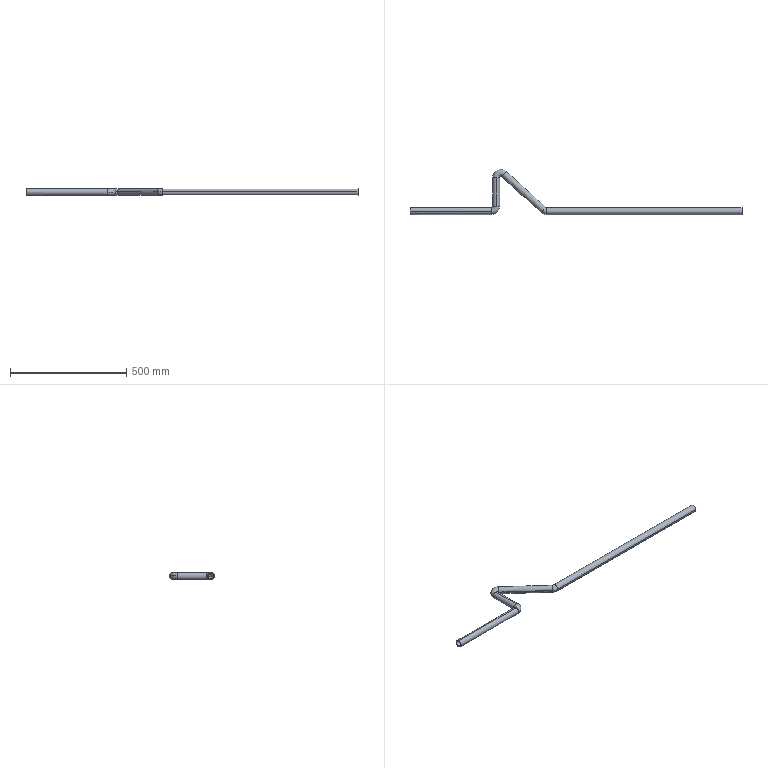Part | SolidWorks | features 3DProfileFeature 2, Sweep 1 | 1 solid | 30 faces | box 1430 x 195.048 x 30 mm | volume 288468 mm3 | cylinder 16 | torus 12 | plane 2 | commonest cylinder face diameters 26 x8 30 x8
STEP:
#1=CARTESIAN_POINT('',(-1540.71,3149.368,100.));
#2=VERTEX_POINT('',#1);
#3=CARTESIAN_POINT('',(-1558.147,3130.082,100.));
#4=VERTEX_POINT('',#3);
#5=CARTESIAN_POINT('',(-1549.428,3139.725,100.));
#6=DIRECTION('',(-0.7418,0.6707,0.));
#7=DIRECTION('',(0.6707,0.7418,0.));
#8=AXIS2_PLACEMENT_3D('',#5,#6,#7);
#9=CIRCLE('',#8,13.);
#10=EDGE_CURVE('',#2,#4,#9,.T.);
#11=ORIENTED_EDGE('',*,*,#10,.T.);
#12=CARTESIAN_POINT('',(-1536.015,3121.56,100.));
#13=VERTEX_POINT('',#12);
#14=CARTESIAN_POINT('',(-1536.015,3154.56,100.));
#15=DIRECTION('',(0.,0.,1.));
#16=DIRECTION('',(0.,-1.,0.));
#17=AXIS2_PLACEMENT_3D('',#14,#15,#16);
#18=CIRCLE('',#17,33.);
#19=EDGE_CURVE('',#4,#13,#18,.T.);
#20=ORIENTED_EDGE('',*,*,#19,.T.);
#21=CARTESIAN_POINT('',(-1536.015,3147.56,100.));
#22=VERTEX_POINT('',#21);
#23=CARTESIAN_POINT('',(-1536.015,3134.56,100.));
#24=DIRECTION('',(-1.,0.,0.));
#25=DIRECTION('',(0.,-1.,0.));
#26=AXIS2_PLACEMENT_3D('',#23,#24,#25);
#27=CIRCLE('',#26,13.);
#28=EDGE_CURVE('',#22,#13,#27,.T.);
#29=ORIENTED_EDGE('',*,*,#28,.F.);
#30=CARTESIAN_POINT('',(-1536.015,3154.56,100.));
#31=DIRECTION('',(0.,0.,1.));
#32=DIRECTION('',(0.,-1.,0.));
#33=AXIS2_PLACEMENT_3D('',#30,#31,#32);
#34=CIRCLE('',#33,7.);
#35=EDGE_CURVE('',#2,#22,#34,.T.);
#36=ORIENTED_EDGE('',*,*,#35,.F.);
#37=EDGE_LOOP('',(#11,#20,#29,#36));
#38=FACE_OUTER_BOUND('',#37,.T.);
#39=CARTESIAN_POINT('',(-1536.015,3154.56,100.));
#40=DIRECTION('',(0.,0.,1.));
#41=DIRECTION('',(0.,-1.,0.));
#42=AXIS2_PLACEMENT_3D('',#39,#40,#41);
#43=TOROIDAL_SURFACE('',#42,20.,13.);
#44=ADVANCED_FACE('',(#38),#43,.F.);
#45=CARTESIAN_POINT('',(-1753.961,3279.608,113.));
#46=VERTEX_POINT('',#45);
#47=CARTESIAN_POINT('',(-1766.961,3279.608,100.));
#48=VERTEX_POINT('',#47);
#49=CARTESIAN_POINT('',(-1753.961,3279.608,100.));
#50=DIRECTION('',(0.,-1.,0.));
#51=DIRECTION('',(0.,0.,1.));
#52=AXIS2_PLACEMENT_3D('',#49,#50,#51);
#53=CIRCLE('',#52,13.);
#54=EDGE_CURVE('',#46,#48,#53,.T.);
#55=ORIENTED_EDGE('',*,*,#54,.T.);
#56=CARTESIAN_POINT('',(-1711.829,3304.086,100.));
#57=VERTEX_POINT('',#56);
#58=CARTESIAN_POINT('',(-1733.961,3279.608,100.));
#59=DIRECTION('',(0.,0.,-1.));
#60=DIRECTION('',(-1.,0.,0.));
#61=AXIS2_PLACEMENT_3D('',#58,#59,#60);
#62=CIRCLE('',#61,33.);
#63=EDGE_CURVE('',#48,#57,#62,.T.);
#64=ORIENTED_EDGE('',*,*,#63,.T.);
#65=CARTESIAN_POINT('',(-1729.266,3284.801,100.));
#66=VERTEX_POINT('',#65);
#67=CARTESIAN_POINT('',(-1720.547,3294.443,100.));
#68=DIRECTION('',(-0.7418,0.6707,0.));
#69=DIRECTION('',(-0.6707,-0.7418,0.));
#70=AXIS2_PLACEMENT_3D('',#67,#68,#69);
#71=CIRCLE('',#70,13.);
#72=EDGE_CURVE('',#66,#57,#71,.T.);
#73=ORIENTED_EDGE('',*,*,#72,.F.);
#74=CARTESIAN_POINT('',(-1740.961,3279.608,100.));
#75=VERTEX_POINT('',#74);
#76=CARTESIAN_POINT('',(-1733.961,3279.608,100.));
#77=DIRECTION('',(0.,0.,-1.));
#78=DIRECTION('',(-1.,0.,0.));
#79=AXIS2_PLACEMENT_3D('',#76,#77,#78);
#80=CIRCLE('',#79,7.);
#81=EDGE_CURVE('',#75,#66,#80,.T.);
#82=ORIENTED_EDGE('',*,*,#81,.F.);
#83=CARTESIAN_POINT('',(-1753.961,3279.608,100.));
#84=DIRECTION('',(0.,-1.,0.));
#85=DIRECTION('',(0.,0.,1.));
#86=AXIS2_PLACEMENT_3D('',#83,#84,#85);
#87=CIRCLE('',#86,13.);
#88=EDGE_CURVE('',#75,#46,#87,.T.);
#89=ORIENTED_EDGE('',*,*,#88,.T.);
#90=EDGE_LOOP('',(#55,#64,#73,#82,#89));
#91=FACE_OUTER_BOUND('',#90,.T.);
#92=CARTESIAN_POINT('',(-1733.961,3279.608,100.));
#93=DIRECTION('',(0.,0.,-1.));
#94=DIRECTION('',(-1.,0.,0.));
#95=AXIS2_PLACEMENT_3D('',#92,#93,#94);
#96=TOROIDAL_SURFACE('',#95,20.,13.);
#97=ADVANCED_FACE('',(#91),#96,.F.);
#98=CARTESIAN_POINT('',(-1773.961,3135.003,87.));
#99=VERTEX_POINT('',#98);
#100=CARTESIAN_POINT('',(-1773.961,3122.003,100.));
#101=VERTEX_POINT('',#100);
#102=CARTESIAN_POINT('',(-1773.961,3135.003,100.));
#103=DIRECTION('',(-1.,0.,0.));
#104=DIRECTION('',(0.,0.,-1.));
#105=AXIS2_PLACEMENT_3D('',#102,#103,#104);
#106=CIRCLE('',#105,13.);
#107=EDGE_CURVE('',#99,#101,#106,.T.);
#108=ORIENTED_EDGE('',*,*,#107,.T.);
#109=CARTESIAN_POINT('',(-1740.961,3155.003,100.));
#110=VERTEX_POINT('',#109);
#111=CARTESIAN_POINT('',(-1773.961,3155.003,100.));
#112=DIRECTION('',(0.,0.,1.));
#113=DIRECTION('',(1.,0.,0.));
#114=AXIS2_PLACEMENT_3D('',#111,#112,#113);
#115=CIRCLE('',#114,33.);
#116=EDGE_CURVE('',#101,#110,#115,.T.);
#117=ORIENTED_EDGE('',*,*,#116,.T.);
#118=CARTESIAN_POINT('',(-1753.961,3155.003,87.));
#119=VERTEX_POINT('',#118);
#120=CARTESIAN_POINT('',(-1753.961,3155.003,100.));
#121=DIRECTION('',(0.,-1.,0.));
#122=DIRECTION('',(0.,0.,-1.));
#123=AXIS2_PLACEMENT_3D('',#120,#121,#122);
#124=CIRCLE('',#123,13.);
#125=EDGE_CURVE('',#119,#110,#124,.T.);
#126=ORIENTED_EDGE('',*,*,#125,.F.);
#127=CARTESIAN_POINT('',(-1766.961,3155.003,100.));
#128=VERTEX_POINT('',#127);
#129=CARTESIAN_POINT('',(-1753.961,3155.003,100.));
#130=DIRECTION('',(0.,-1.,0.));
#131=DIRECTION('',(0.,0.,-1.));
#132=AXIS2_PLACEMENT_3D('',#129,#130,#131);
#133=CIRCLE('',#132,13.);
#134=EDGE_CURVE('',#128,#119,#133,.T.);
#135=ORIENTED_EDGE('',*,*,#134,.F.);
#136=CARTESIAN_POINT('',(-1773.961,3148.003,100.));
#137=VERTEX_POINT('',#136);
#138=CARTESIAN_POINT('',(-1773.961,3155.003,100.));
#139=DIRECTION('',(0.,0.,1.));
#140=DIRECTION('',(1.,0.,0.));
#141=AXIS2_PLACEMENT_3D('',#138,#139,#140);
#142=CIRCLE('',#141,7.);
#143=EDGE_CURVE('',#137,#128,#142,.T.);
#144=ORIENTED_EDGE('',*,*,#143,.F.);
#145=CARTESIAN_POINT('',(-1773.961,3135.003,100.));
#146=DIRECTION('',(-1.,0.,0.));
#147=DIRECTION('',(0.,0.,-1.));
#148=AXIS2_PLACEMENT_3D('',#145,#146,#147);
#149=CIRCLE('',#148,13.);
#150=EDGE_CURVE('',#137,#99,#149,.T.);
#151=ORIENTED_EDGE('',*,*,#150,.T.);
#152=EDGE_LOOP('',(#108,#117,#126,#135,#144,#151));
#153=FACE_OUTER_BOUND('',#152,.T.);
#154=CARTESIAN_POINT('',(-1773.961,3155.003,100.));
#155=DIRECTION('',(0.,0.,1.));
#156=DIRECTION('',(1.,0.,0.));
#157=AXIS2_PLACEMENT_3D('',#154,#155,#156);
#158=TOROIDAL_SURFACE('',#157,20.,13.);
#159=ADVANCED_FACE('',(#153),#158,.F.);
#160=CARTESIAN_POINT('',(-1559.488,3128.598,100.));
#161=VERTEX_POINT('',#160);
#162=CARTESIAN_POINT('',(-1539.368,3150.851,100.));
#163=VERTEX_POINT('',#162);
#164=CARTESIAN_POINT('',(-1549.428,3139.725,100.));
#165=DIRECTION('',(-0.7418,0.6707,0.));
#166=DIRECTION('',(0.,0.,1.));
#167=AXIS2_PLACEMENT_3D('',#164,#165,#166);
#168=CIRCLE('',#167,15.);
#169=EDGE_CURVE('',#161,#163,#168,.T.);
#170=ORIENTED_EDGE('',*,*,#169,.F.);
#171=CARTESIAN_POINT('',(-1536.015,3119.56,100.));
#172=VERTEX_POINT('',#171);
#173=CARTESIAN_POINT('',(-1536.015,3154.56,100.));
#174=DIRECTION('',(0.,0.,1.));
#175=DIRECTION('',(0.,-1.,0.));
#176=AXIS2_PLACEMENT_3D('',#173,#174,#175);
#177=CIRCLE('',#176,35.);
#178=EDGE_CURVE('',#161,#172,#177,.T.);
#179=ORIENTED_EDGE('',*,*,#178,.T.);
#180=CARTESIAN_POINT('',(-1536.015,3149.56,100.));
#181=VERTEX_POINT('',#180);
#182=CARTESIAN_POINT('',(-1536.015,3134.56,100.));
#183=DIRECTION('',(-1.,0.,0.));
#184=DIRECTION('',(0.,0.,1.));
#185=AXIS2_PLACEMENT_3D('',#182,#183,#184);
#186=CIRCLE('',#185,15.);
#187=EDGE_CURVE('',#172,#181,#186,.T.);
#188=ORIENTED_EDGE('',*,*,#187,.T.);
#189=CARTESIAN_POINT('',(-1536.015,3154.56,100.));
#190=DIRECTION('',(0.,0.,1.));
#191=DIRECTION('',(0.,-1.,0.));
#192=AXIS2_PLACEMENT_3D('',#189,#190,#191);
#193=CIRCLE('',#192,5.);
#194=EDGE_CURVE('',#163,#181,#193,.T.);
#195=ORIENTED_EDGE('',*,*,#194,.F.);
#196=EDGE_LOOP('',(#170,#179,#188,#195));
#197=FACE_OUTER_BOUND('',#196,.T.);
#198=CARTESIAN_POINT('',(-1536.015,3154.56,100.));
#199=DIRECTION('',(0.,0.,1.));
#200=DIRECTION('',(0.,-1.,0.));
#201=AXIS2_PLACEMENT_3D('',#198,#199,#200);
#202=TOROIDAL_SURFACE('',#201,20.,15.);
#203=ADVANCED_FACE('',(#197),#202,.T.);
#204=CARTESIAN_POINT('',(-1768.961,3279.608,100.));
#205=VERTEX_POINT('',#204);
#206=CARTESIAN_POINT('',(-1753.961,3279.608,85.));
#207=VERTEX_POINT('',#206);
#208=CARTESIAN_POINT('',(-1753.961,3279.608,100.));
#209=DIRECTION('',(0.,-1.,0.));
#210=DIRECTION('',(0.,0.,1.));
#211=AXIS2_PLACEMENT_3D('',#208,#209,#210);
#212=CIRCLE('',#211,15.);
#213=EDGE_CURVE('',#205,#207,#212,.T.);
#214=ORIENTED_EDGE('',*,*,#213,.F.);
#215=CARTESIAN_POINT('',(-1710.487,3305.57,100.));
#216=VERTEX_POINT('',#215);
#217=CARTESIAN_POINT('',(-1733.961,3279.608,100.));
#218=DIRECTION('',(0.,0.,-1.));
#219=DIRECTION('',(-1.,0.,0.));
#220=AXIS2_PLACEMENT_3D('',#217,#218,#219);
#221=CIRCLE('',#220,35.);
#222=EDGE_CURVE('',#205,#216,#221,.T.);
#223=ORIENTED_EDGE('',*,*,#222,.T.);
#224=CARTESIAN_POINT('',(-1730.607,3283.317,100.));
#225=VERTEX_POINT('',#224);
#226=CARTESIAN_POINT('',(-1720.547,3294.443,100.));
#227=DIRECTION('',(-0.7418,0.6707,0.));
#228=DIRECTION('',(0.,0.,1.));
#229=AXIS2_PLACEMENT_3D('',#226,#227,#228);
#230=CIRCLE('',#229,15.);
#231=EDGE_CURVE('',#216,#225,#230,.T.);
#232=ORIENTED_EDGE('',*,*,#231,.T.);
#233=CARTESIAN_POINT('',(-1738.961,3279.608,100.));
#234=VERTEX_POINT('',#233);
#235=CARTESIAN_POINT('',(-1733.961,3279.608,100.));
#236=DIRECTION('',(0.,0.,-1.));
#237=DIRECTION('',(-1.,0.,0.));
#238=AXIS2_PLACEMENT_3D('',#235,#236,#237);
#239=CIRCLE('',#238,5.);
#240=EDGE_CURVE('',#234,#225,#239,.T.);
#241=ORIENTED_EDGE('',*,*,#240,.F.);
#242=CARTESIAN_POINT('',(-1753.961,3279.608,100.));
#243=DIRECTION('',(0.,-1.,0.));
#244=DIRECTION('',(0.,0.,1.));
#245=AXIS2_PLACEMENT_3D('',#242,#243,#244);
#246=CIRCLE('',#245,15.);
#247=EDGE_CURVE('',#207,#234,#246,.T.);
#248=ORIENTED_EDGE('',*,*,#247,.F.);
#249=EDGE_LOOP('',(#214,#223,#232,#241,#248));
#250=FACE_OUTER_BOUND('',#249,.T.);
#251=CARTESIAN_POINT('',(-1733.961,3279.608,100.));
#252=DIRECTION('',(0.,0.,-1.));
#253=DIRECTION('',(-1.,0.,0.));
#254=AXIS2_PLACEMENT_3D('',#251,#252,#253);
#255=TOROIDAL_SURFACE('',#254,20.,15.);
#256=ADVANCED_FACE('',(#250),#255,.T.);
#257=CARTESIAN_POINT('',(-1773.961,3120.003,100.));
#258=VERTEX_POINT('',#257);
#259=CARTESIAN_POINT('',(-1773.961,3135.003,115.));
#260=VERTEX_POINT('',#259);
#261=CARTESIAN_POINT('',(-1773.961,3135.003,100.));
#262=DIRECTION('',(-1.,0.,0.));
#263=DIRECTION('',(0.,0.,1.));
#264=AXIS2_PLACEMENT_3D('',#261,#262,#263);
#265=CIRCLE('',#264,15.);
#266=EDGE_CURVE('',#258,#260,#265,.T.);
#267=ORIENTED_EDGE('',*,*,#266,.F.);
#268=CARTESIAN_POINT('',(-1738.961,3155.003,100.));
#269=VERTEX_POINT('',#268);
#270=CARTESIAN_POINT('',(-1773.961,3155.003,100.));
#271=DIRECTION('',(0.,0.,1.));
#272=DIRECTION('',(1.,0.,0.));
#273=AXIS2_PLACEMENT_3D('',#270,#271,#272);
#274=CIRCLE('',#273,35.);
#275=EDGE_CURVE('',#258,#269,#274,.T.);
#276=ORIENTED_EDGE('',*,*,#275,.T.);
#277=CARTESIAN_POINT('',(-1753.961,3155.003,115.));
#278=VERTEX_POINT('',#277);
#279=CARTESIAN_POINT('',(-1753.961,3155.003,100.));
#280=DIRECTION('',(0.,-1.,0.));
#281=DIRECTION('',(0.,0.,1.));
#282=AXIS2_PLACEMENT_3D('',#279,#280,#281);
#283=CIRCLE('',#282,15.);
#284=EDGE_CURVE('',#269,#278,#283,.T.);
#285=ORIENTED_EDGE('',*,*,#284,.T.);
#286=CARTESIAN_POINT('',(-1768.961,3155.003,100.));
#287=VERTEX_POINT('',#286);
#288=CARTESIAN_POINT('',(-1753.961,3155.003,100.));
#289=DIRECTION('',(0.,-1.,0.));
#290=DIRECTION('',(0.,0.,1.));
#291=AXIS2_PLACEMENT_3D('',#288,#289,#290);
#292=CIRCLE('',#291,15.);
#293=EDGE_CURVE('',#278,#287,#292,.T.);
#294=ORIENTED_EDGE('',*,*,#293,.T.);
#295=CARTESIAN_POINT('',(-1773.961,3150.003,100.));
#296=VERTEX_POINT('',#295);
#297=CARTESIAN_POINT('',(-1773.961,3155.003,100.));
#298=DIRECTION('',(0.,0.,1.));
#299=DIRECTION('',(1.,0.,0.));
#300=AXIS2_PLACEMENT_3D('',#297,#298,#299);
#301=CIRCLE('',#300,5.);
#302=EDGE_CURVE('',#296,#287,#301,.T.);
#303=ORIENTED_EDGE('',*,*,#302,.F.);
#304=CARTESIAN_POINT('',(-1773.961,3135.003,100.));
#305=DIRECTION('',(-1.,0.,0.));
#306=DIRECTION('',(0.,0.,1.));
#307=AXIS2_PLACEMENT_3D('',#304,#305,#306);
#308=CIRCLE('',#307,15.);
#309=EDGE_CURVE('',#260,#296,#308,.T.);
#310=ORIENTED_EDGE('',*,*,#309,.F.);
#311=EDGE_LOOP('',(#267,#276,#285,#294,#303,#310));
#312=FACE_OUTER_BOUND('',#311,.T.);
#313=CARTESIAN_POINT('',(-1773.961,3155.003,100.));
#314=DIRECTION('',(0.,0.,1.));
#315=DIRECTION('',(1.,0.,0.));
#316=AXIS2_PLACEMENT_3D('',#313,#314,#315);
#317=TOROIDAL_SURFACE('',#316,20.,15.);
#318=ADVANCED_FACE('',(#312),#317,.T.);
#319=ORIENTED_EDGE('',*,*,#28,.T.);
#320=CARTESIAN_POINT('',(-694.91,3121.56,100.));
#321=VERTEX_POINT('',#320);
#322=CARTESIAN_POINT('',(-1536.015,3121.56,100.));
#323=DIRECTION('',(1.,0.,0.));
#324=VECTOR('',#323,1000.);
#325=LINE('',#322,#324);
#326=EDGE_CURVE('',#13,#321,#325,.T.);
#327=ORIENTED_EDGE('',*,*,#326,.T.);
#328=CARTESIAN_POINT('',(-694.91,3147.56,100.));
#329=VERTEX_POINT('',#328);
#330=CARTESIAN_POINT('',(-694.91,3134.56,100.));
#331=DIRECTION('',(-1.,0.,0.));
#332=DIRECTION('',(0.,0.,1.));
#333=AXIS2_PLACEMENT_3D('',#330,#331,#332);
#334=CIRCLE('',#333,13.);
#335=EDGE_CURVE('',#329,#321,#334,.T.);
#336=ORIENTED_EDGE('',*,*,#335,.F.);
#337=CARTESIAN_POINT('',(-1536.015,3147.56,100.));
#338=DIRECTION('',(1.,0.,0.));
#339=VECTOR('',#338,1000.);
#340=LINE('',#337,#339);
#341=EDGE_CURVE('',#22,#329,#340,.T.);
#342=ORIENTED_EDGE('',*,*,#341,.F.);
#343=EDGE_LOOP('',(#319,#327,#336,#342));
#344=FACE_OUTER_BOUND('',#343,.T.);
#345=CARTESIAN_POINT('',(-1536.015,3134.56,100.));
#346=DIRECTION('',(1.,0.,0.));
#347=DIRECTION('',(0.,1.,0.));
#348=AXIS2_PLACEMENT_3D('',#345,#346,#347);
#349=CYLINDRICAL_SURFACE('',#348,13.);
#350=ADVANCED_FACE('',(#344),#349,.F.);
#351=CARTESIAN_POINT('',(-1720.547,3294.443,100.));
#352=DIRECTION('',(-0.7418,0.6707,0.));
#353=DIRECTION('',(-0.6707,-0.7418,0.));
#354=AXIS2_PLACEMENT_3D('',#351,#352,#353);
#355=CIRCLE('',#354,13.);
#356=EDGE_CURVE('',#57,#66,#355,.T.);
#357=ORIENTED_EDGE('',*,*,#356,.T.);
#358=CARTESIAN_POINT('',(-1729.266,3284.801,100.));
#359=DIRECTION('',(0.7418,-0.6707,0.));
#360=VECTOR('',#359,1000.);
#361=LINE('',#358,#360);
#362=EDGE_CURVE('',#66,#4,#361,.T.);
#363=ORIENTED_EDGE('',*,*,#362,.T.);
#364=ORIENTED_EDGE('',*,*,#10,.F.);
#365=CARTESIAN_POINT('',(-1711.829,3304.086,100.));
#366=DIRECTION('',(0.7418,-0.6707,0.));
#367=VECTOR('',#366,1000.);
#368=LINE('',#365,#367);
#369=EDGE_CURVE('',#57,#2,#368,.T.);
#370=ORIENTED_EDGE('',*,*,#369,.F.);
#371=EDGE_LOOP('',(#357,#363,#364,#370));
#372=FACE_OUTER_BOUND('',#371,.T.);
#373=CARTESIAN_POINT('',(-1720.547,3294.443,100.));
#374=DIRECTION('',(0.7418,-0.6707,0.));
#375=DIRECTION('',(0.6707,0.7418,0.));
#376=AXIS2_PLACEMENT_3D('',#373,#374,#375);
#377=CYLINDRICAL_SURFACE('',#376,13.);
#378=ADVANCED_FACE('',(#372),#377,.F.);
#379=CARTESIAN_POINT('',(-1753.961,3155.003,113.));
#380=VERTEX_POINT('',#379);
#381=CARTESIAN_POINT('',(-1753.961,3155.003,100.));
#382=DIRECTION('',(0.,-1.,0.));
#383=DIRECTION('',(0.,0.,-1.));
#384=AXIS2_PLACEMENT_3D('',#381,#382,#383);
#385=CIRCLE('',#384,13.);
#386=EDGE_CURVE('',#380,#128,#385,.T.);
#387=ORIENTED_EDGE('',*,*,#386,.T.);
#388=ORIENTED_EDGE('',*,*,#134,.T.);
#389=CARTESIAN_POINT('',(-1753.961,3279.608,87.));
#390=VERTEX_POINT('',#389);
#391=CARTESIAN_POINT('',(-1753.961,3155.003,87.));
#392=DIRECTION('',(0.,1.,0.));
#393=VECTOR('',#392,1000.);
#394=LINE('',#391,#393);
#395=EDGE_CURVE('',#119,#390,#394,.T.);
#396=ORIENTED_EDGE('',*,*,#395,.T.);
#397=CARTESIAN_POINT('',(-1753.961,3279.608,100.));
#398=DIRECTION('',(0.,-1.,0.));
#399=DIRECTION('',(0.,0.,1.));
#400=AXIS2_PLACEMENT_3D('',#397,#398,#399);
#401=CIRCLE('',#400,13.);
#402=EDGE_CURVE('',#48,#390,#401,.T.);
#403=ORIENTED_EDGE('',*,*,#402,.F.);
#404=ORIENTED_EDGE('',*,*,#54,.F.);
#405=CARTESIAN_POINT('',(-1753.961,3155.003,113.));
#406=DIRECTION('',(0.,1.,0.));
#407=VECTOR('',#406,1000.);
#408=LINE('',#405,#407);
#409=EDGE_CURVE('',#380,#46,#408,.T.);
#410=ORIENTED_EDGE('',*,*,#409,.F.);
#411=EDGE_LOOP('',(#387,#388,#396,#403,#404,#410));
#412=FACE_OUTER_BOUND('',#411,.T.);
#413=CARTESIAN_POINT('',(-1753.961,3155.003,100.));
#414=DIRECTION('',(0.,1.,0.));
#415=DIRECTION('',(0.,0.,1.));
#416=AXIS2_PLACEMENT_3D('',#413,#414,#415);
#417=CYLINDRICAL_SURFACE('',#416,13.);
#418=ADVANCED_FACE('',(#412),#417,.F.);
#419=CARTESIAN_POINT('',(-2125.,3135.003,87.));
#420=VERTEX_POINT('',#419);
#421=CARTESIAN_POINT('',(-2125.,3135.003,113.));
#422=VERTEX_POINT('',#421);
#423=CARTESIAN_POINT('',(-2125.,3135.003,100.));
#424=DIRECTION('',(-1.,0.,0.));
#425=DIRECTION('',(0.,0.,1.));
#426=AXIS2_PLACEMENT_3D('',#423,#424,#425);
#427=CIRCLE('',#426,13.);
#428=EDGE_CURVE('',#420,#422,#427,.T.);
#429=ORIENTED_EDGE('',*,*,#428,.T.);
#430=CARTESIAN_POINT('',(-1773.961,3135.003,113.));
#431=VERTEX_POINT('',#430);
#432=CARTESIAN_POINT('',(-2125.,3135.003,113.));
#433=DIRECTION('',(1.,0.,0.));
#434=VECTOR('',#433,1000.);
#435=LINE('',#432,#434);
#436=EDGE_CURVE('',#422,#431,#435,.T.);
#437=ORIENTED_EDGE('',*,*,#436,.T.);
#438=CARTESIAN_POINT('',(-1773.961,3135.003,100.));
#439=DIRECTION('',(-1.,0.,0.));
#440=DIRECTION('',(0.,0.,-1.));
#441=AXIS2_PLACEMENT_3D('',#438,#439,#440);
#442=CIRCLE('',#441,13.);
#443=EDGE_CURVE('',#101,#431,#442,.T.);
#444=ORIENTED_EDGE('',*,*,#443,.F.);
#445=ORIENTED_EDGE('',*,*,#107,.F.);
#446=CARTESIAN_POINT('',(-2125.,3135.003,87.));
#447=DIRECTION('',(1.,0.,0.));
#448=VECTOR('',#447,1000.);
#449=LINE('',#446,#448);
#450=EDGE_CURVE('',#420,#99,#449,.T.);
#451=ORIENTED_EDGE('',*,*,#450,.F.);
#452=EDGE_LOOP('',(#429,#437,#444,#445,#451));
#453=FACE_OUTER_BOUND('',#452,.T.);
#454=CARTESIAN_POINT('',(-2125.,3135.003,100.));
#455=DIRECTION('',(1.,0.,0.));
#456=DIRECTION('',(0.,0.,-1.));
#457=AXIS2_PLACEMENT_3D('',#454,#455,#456);
#458=CYLINDRICAL_SURFACE('',#457,13.);
#459=ADVANCED_FACE('',(#453),#458,.F.);
#460=ORIENTED_EDGE('',*,*,#187,.F.);
#461=CARTESIAN_POINT('',(-694.91,3119.56,100.));
#462=VERTEX_POINT('',#461);
#463=CARTESIAN_POINT('',(-1536.015,3119.56,100.));
#464=DIRECTION('',(1.,0.,0.));
#465=VECTOR('',#464,1000.);
#466=LINE('',#463,#465);
#467=EDGE_CURVE('',#172,#462,#466,.T.);
#468=ORIENTED_EDGE('',*,*,#467,.T.);
#469=CARTESIAN_POINT('',(-694.91,3149.56,100.));
#470=VERTEX_POINT('',#469);
#471=CARTESIAN_POINT('',(-694.91,3134.56,100.));
#472=DIRECTION('',(-1.,0.,0.));
#473=DIRECTION('',(0.,0.,1.));
#474=AXIS2_PLACEMENT_3D('',#471,#472,#473);
#475=CIRCLE('',#474,15.);
#476=EDGE_CURVE('',#462,#470,#475,.T.);
#477=ORIENTED_EDGE('',*,*,#476,.T.);
#478=CARTESIAN_POINT('',(-1536.015,3149.56,100.));
#479=DIRECTION('',(1.,0.,0.));
#480=VECTOR('',#479,1000.);
#481=LINE('',#478,#480);
#482=EDGE_CURVE('',#181,#470,#481,.T.);
#483=ORIENTED_EDGE('',*,*,#482,.F.);
#484=EDGE_LOOP('',(#460,#468,#477,#483));
#485=FACE_OUTER_BOUND('',#484,.T.);
#486=CARTESIAN_POINT('',(-1536.015,3134.56,100.));
#487=DIRECTION('',(1.,0.,0.));
#488=DIRECTION('',(0.,1.,0.));
#489=AXIS2_PLACEMENT_3D('',#486,#487,#488);
#490=CYLINDRICAL_SURFACE('',#489,15.);
#491=ADVANCED_FACE('',(#485),#490,.T.);
#492=CARTESIAN_POINT('',(-1720.547,3294.443,100.));
#493=DIRECTION('',(-0.7418,0.6707,0.));
#494=DIRECTION('',(0.,0.,1.));
#495=AXIS2_PLACEMENT_3D('',#492,#493,#494);
#496=CIRCLE('',#495,15.);
#497=EDGE_CURVE('',#225,#216,#496,.T.);
#498=ORIENTED_EDGE('',*,*,#497,.F.);
#499=CARTESIAN_POINT('',(-1730.607,3283.317,100.));
#500=DIRECTION('',(0.7418,-0.6707,0.));
#501=VECTOR('',#500,1000.);
#502=LINE('',#499,#501);
#503=EDGE_CURVE('',#225,#161,#502,.T.);
#504=ORIENTED_EDGE('',*,*,#503,.T.);
#505=ORIENTED_EDGE('',*,*,#169,.T.);
#506=CARTESIAN_POINT('',(-1710.487,3305.57,100.));
#507=DIRECTION('',(0.7418,-0.6707,0.));
#508=VECTOR('',#507,1000.);
#509=LINE('',#506,#508);
#510=EDGE_CURVE('',#216,#163,#509,.T.);
#511=ORIENTED_EDGE('',*,*,#510,.F.);
#512=EDGE_LOOP('',(#498,#504,#505,#511));
#513=FACE_OUTER_BOUND('',#512,.T.);
#514=CARTESIAN_POINT('',(-1720.547,3294.443,100.));
#515=DIRECTION('',(0.7418,-0.6707,0.));
#516=DIRECTION('',(0.6707,0.7418,0.));
#517=AXIS2_PLACEMENT_3D('',#514,#515,#516);
#518=CYLINDRICAL_SURFACE('',#517,15.);
#519=ADVANCED_FACE('',(#513),#518,.T.);
#520=CARTESIAN_POINT('',(-1753.961,3155.003,85.));
#521=VERTEX_POINT('',#520);
#522=CARTESIAN_POINT('',(-1753.961,3155.003,100.));
#523=DIRECTION('',(0.,-1.,0.));
#524=DIRECTION('',(0.,0.,1.));
#525=AXIS2_PLACEMENT_3D('',#522,#523,#524);
#526=CIRCLE('',#525,15.);
#527=EDGE_CURVE('',#521,#269,#526,.T.);
#528=ORIENTED_EDGE('',*,*,#527,.F.);
#529=CARTESIAN_POINT('',(-1753.961,3155.003,85.));
#530=DIRECTION('',(0.,1.,0.));
#531=VECTOR('',#530,1000.);
#532=LINE('',#529,#531);
#533=EDGE_CURVE('',#521,#207,#532,.T.);
#534=ORIENTED_EDGE('',*,*,#533,.T.);
#535=ORIENTED_EDGE('',*,*,#247,.T.);
#536=CARTESIAN_POINT('',(-1753.961,3279.608,115.));
#537=VERTEX_POINT('',#536);
#538=CARTESIAN_POINT('',(-1753.961,3279.608,100.));
#539=DIRECTION('',(0.,-1.,0.));
#540=DIRECTION('',(0.,0.,1.));
#541=AXIS2_PLACEMENT_3D('',#538,#539,#540);
#542=CIRCLE('',#541,15.);
#543=EDGE_CURVE('',#234,#537,#542,.T.);
#544=ORIENTED_EDGE('',*,*,#543,.T.);
#545=CARTESIAN_POINT('',(-1753.961,3155.003,115.));
#546=DIRECTION('',(0.,1.,0.));
#547=VECTOR('',#546,1000.);
#548=LINE('',#545,#547);
#549=EDGE_CURVE('',#278,#537,#548,.T.);
#550=ORIENTED_EDGE('',*,*,#549,.F.);
#551=ORIENTED_EDGE('',*,*,#284,.F.);
#552=EDGE_LOOP('',(#528,#534,#535,#544,#550,#551));
#553=FACE_OUTER_BOUND('',#552,.T.);
#554=CARTESIAN_POINT('',(-1753.961,3155.003,100.));
#555=DIRECTION('',(0.,1.,0.));
#556=DIRECTION('',(0.,0.,1.));
#557=AXIS2_PLACEMENT_3D('',#554,#555,#556);
#558=CYLINDRICAL_SURFACE('',#557,15.);
#559=ADVANCED_FACE('',(#553),#558,.T.);
#560=CARTESIAN_POINT('',(-2125.,3135.003,115.));
#561=VERTEX_POINT('',#560);
#562=CARTESIAN_POINT('',(-2125.,3135.003,85.));
#563=VERTEX_POINT('',#562);
#564=CARTESIAN_POINT('',(-2125.,3135.003,100.));
#565=DIRECTION('',(-1.,0.,0.));
#566=DIRECTION('',(0.,0.,1.));
#567=AXIS2_PLACEMENT_3D('',#564,#565,#566);
#568=CIRCLE('',#567,15.);
#569=EDGE_CURVE('',#561,#563,#568,.T.);
#570=ORIENTED_EDGE('',*,*,#569,.F.);
#571=CARTESIAN_POINT('',(-2125.,3135.003,115.));
#572=DIRECTION('',(1.,0.,0.));
#573=VECTOR('',#572,1000.);
#574=LINE('',#571,#573);
#575=EDGE_CURVE('',#561,#260,#574,.T.);
#576=ORIENTED_EDGE('',*,*,#575,.T.);
#577=ORIENTED_EDGE('',*,*,#309,.T.);
#578=CARTESIAN_POINT('',(-1773.961,3135.003,85.));
#579=VERTEX_POINT('',#578);
#580=CARTESIAN_POINT('',(-1773.961,3135.003,100.));
#581=DIRECTION('',(-1.,0.,0.));
#582=DIRECTION('',(0.,0.,1.));
#583=AXIS2_PLACEMENT_3D('',#580,#581,#582);
#584=CIRCLE('',#583,15.);
#585=EDGE_CURVE('',#296,#579,#584,.T.);
#586=ORIENTED_EDGE('',*,*,#585,.T.);
#587=CARTESIAN_POINT('',(-2125.,3135.003,85.));
#588=DIRECTION('',(1.,0.,0.));
#589=VECTOR('',#588,1000.);
#590=LINE('',#587,#589);
#591=EDGE_CURVE('',#563,#579,#590,.T.);
#592=ORIENTED_EDGE('',*,*,#591,.F.);
#593=EDGE_LOOP('',(#570,#576,#577,#586,#592));
#594=FACE_OUTER_BOUND('',#593,.T.);
#595=CARTESIAN_POINT('',(-2125.,3135.003,100.));
#596=DIRECTION('',(1.,0.,0.));
#597=DIRECTION('',(0.,0.,-1.));
#598=AXIS2_PLACEMENT_3D('',#595,#596,#597);
#599=CYLINDRICAL_SURFACE('',#598,15.);
#600=ADVANCED_FACE('',(#594),#599,.T.);
#601=ORIENTED_EDGE('',*,*,#467,.F.);
#602=CARTESIAN_POINT('',(-1536.015,3134.56,100.));
#603=DIRECTION('',(-1.,0.,0.));
#604=DIRECTION('',(0.,0.,1.));
#605=AXIS2_PLACEMENT_3D('',#602,#603,#604);
#606=CIRCLE('',#605,15.);
#607=EDGE_CURVE('',#181,#172,#606,.T.);
#608=ORIENTED_EDGE('',*,*,#607,.F.);
#609=ORIENTED_EDGE('',*,*,#482,.T.);
#610=CARTESIAN_POINT('',(-694.91,3134.56,100.));
#611=DIRECTION('',(-1.,0.,0.));
#612=DIRECTION('',(0.,0.,1.));
#613=AXIS2_PLACEMENT_3D('',#610,#611,#612);
#614=CIRCLE('',#613,15.);
#615=EDGE_CURVE('',#470,#462,#614,.T.);
#616=ORIENTED_EDGE('',*,*,#615,.T.);
#617=EDGE_LOOP('',(#601,#608,#609,#616));
#618=FACE_OUTER_BOUND('',#617,.T.);
#619=CARTESIAN_POINT('',(-1536.015,3134.56,100.));
#620=DIRECTION('',(1.,0.,0.));
#621=DIRECTION('',(0.,1.,0.));
#622=AXIS2_PLACEMENT_3D('',#619,#620,#621);
#623=CYLINDRICAL_SURFACE('',#622,15.);
#624=ADVANCED_FACE('',(#618),#623,.T.);
#625=ORIENTED_EDGE('',*,*,#178,.F.);
#626=CARTESIAN_POINT('',(-1549.428,3139.725,100.));
#627=DIRECTION('',(-0.7418,0.6707,0.));
#628=DIRECTION('',(0.,0.,1.));
#629=AXIS2_PLACEMENT_3D('',#626,#627,#628);
#630=CIRCLE('',#629,15.);
#631=EDGE_CURVE('',#163,#161,#630,.T.);
#632=ORIENTED_EDGE('',*,*,#631,.F.);
#633=ORIENTED_EDGE('',*,*,#194,.T.);
#634=ORIENTED_EDGE('',*,*,#607,.T.);
#635=EDGE_LOOP('',(#625,#632,#633,#634));
#636=FACE_OUTER_BOUND('',#635,.T.);
#637=CARTESIAN_POINT('',(-1536.015,3154.56,100.));
#638=DIRECTION('',(0.,0.,1.));
#639=DIRECTION('',(0.,-1.,0.));
#640=AXIS2_PLACEMENT_3D('',#637,#638,#639);
#641=TOROIDAL_SURFACE('',#640,20.,15.);
#642=ADVANCED_FACE('',(#636),#641,.T.);
#643=ORIENTED_EDGE('',*,*,#503,.F.);
#644=ORIENTED_EDGE('',*,*,#231,.F.);
#645=ORIENTED_EDGE('',*,*,#510,.T.);
#646=ORIENTED_EDGE('',*,*,#631,.T.);
#647=EDGE_LOOP('',(#643,#644,#645,#646));
#648=FACE_OUTER_BOUND('',#647,.T.);
#649=CARTESIAN_POINT('',(-1720.547,3294.443,100.));
#650=DIRECTION('',(0.7418,-0.6707,0.));
#651=DIRECTION('',(0.6707,0.7418,0.));
#652=AXIS2_PLACEMENT_3D('',#649,#650,#651);
#653=CYLINDRICAL_SURFACE('',#652,15.);
#654=ADVANCED_FACE('',(#648),#653,.T.);
#655=ORIENTED_EDGE('',*,*,#222,.F.);
#656=CARTESIAN_POINT('',(-1753.961,3279.608,100.));
#657=DIRECTION('',(0.,-1.,0.));
#658=DIRECTION('',(0.,0.,1.));
#659=AXIS2_PLACEMENT_3D('',#656,#657,#658);
#660=CIRCLE('',#659,15.);
#661=EDGE_CURVE('',#537,#205,#660,.T.);
#662=ORIENTED_EDGE('',*,*,#661,.F.);
#663=ORIENTED_EDGE('',*,*,#543,.F.);
#664=ORIENTED_EDGE('',*,*,#240,.T.);
#665=ORIENTED_EDGE('',*,*,#497,.T.);
#666=EDGE_LOOP('',(#655,#662,#663,#664,#665));
#667=FACE_OUTER_BOUND('',#666,.T.);
#668=CARTESIAN_POINT('',(-1733.961,3279.608,100.));
#669=DIRECTION('',(0.,0.,-1.));
#670=DIRECTION('',(-1.,0.,0.));
#671=AXIS2_PLACEMENT_3D('',#668,#669,#670);
#672=TOROIDAL_SURFACE('',#671,20.,15.);
#673=ADVANCED_FACE('',(#667),#672,.T.);
#674=ORIENTED_EDGE('',*,*,#533,.F.);
#675=CARTESIAN_POINT('',(-1753.961,3155.003,100.));
#676=DIRECTION('',(0.,-1.,0.));
#677=DIRECTION('',(0.,0.,1.));
#678=AXIS2_PLACEMENT_3D('',#675,#676,#677);
#679=CIRCLE('',#678,15.);
#680=EDGE_CURVE('',#287,#521,#679,.T.);
#681=ORIENTED_EDGE('',*,*,#680,.F.);
#682=ORIENTED_EDGE('',*,*,#293,.F.);
#683=ORIENTED_EDGE('',*,*,#549,.T.);
#684=ORIENTED_EDGE('',*,*,#661,.T.);
#685=ORIENTED_EDGE('',*,*,#213,.T.);
#686=EDGE_LOOP('',(#674,#681,#682,#683,#684,#685));
#687=FACE_OUTER_BOUND('',#686,.T.);
#688=CARTESIAN_POINT('',(-1753.961,3155.003,100.));
#689=DIRECTION('',(0.,1.,0.));
#690=DIRECTION('',(0.,0.,1.));
#691=AXIS2_PLACEMENT_3D('',#688,#689,#690);
#692=CYLINDRICAL_SURFACE('',#691,15.);
#693=ADVANCED_FACE('',(#687),#692,.T.);
#694=ORIENTED_EDGE('',*,*,#275,.F.);
#695=CARTESIAN_POINT('',(-1773.961,3135.003,100.));
#696=DIRECTION('',(-1.,0.,0.));
#697=DIRECTION('',(0.,0.,1.));
#698=AXIS2_PLACEMENT_3D('',#695,#696,#697);
#699=CIRCLE('',#698,15.);
#700=EDGE_CURVE('',#579,#258,#699,.T.);
#701=ORIENTED_EDGE('',*,*,#700,.F.);
#702=ORIENTED_EDGE('',*,*,#585,.F.);
#703=ORIENTED_EDGE('',*,*,#302,.T.);
#704=ORIENTED_EDGE('',*,*,#680,.T.);
#705=ORIENTED_EDGE('',*,*,#527,.T.);
#706=EDGE_LOOP('',(#694,#701,#702,#703,#704,#705));
#707=FACE_OUTER_BOUND('',#706,.T.);
#708=CARTESIAN_POINT('',(-1773.961,3155.003,100.));
#709=DIRECTION('',(0.,0.,1.));
#710=DIRECTION('',(1.,0.,0.));
#711=AXIS2_PLACEMENT_3D('',#708,#709,#710);
#712=TOROIDAL_SURFACE('',#711,20.,15.);
#713=ADVANCED_FACE('',(#707),#712,.T.);
#714=ORIENTED_EDGE('',*,*,#575,.F.);
#715=CARTESIAN_POINT('',(-2125.,3135.003,100.));
#716=DIRECTION('',(-1.,0.,0.));
#717=DIRECTION('',(0.,0.,1.));
#718=AXIS2_PLACEMENT_3D('',#715,#716,#717);
#719=CIRCLE('',#718,15.);
#720=EDGE_CURVE('',#563,#561,#719,.T.);
#721=ORIENTED_EDGE('',*,*,#720,.F.);
#722=ORIENTED_EDGE('',*,*,#591,.T.);
#723=ORIENTED_EDGE('',*,*,#700,.T.);
#724=ORIENTED_EDGE('',*,*,#266,.T.);
#725=EDGE_LOOP('',(#714,#721,#722,#723,#724));
#726=FACE_OUTER_BOUND('',#725,.T.);
#727=CARTESIAN_POINT('',(-2125.,3135.003,100.));
#728=DIRECTION('',(1.,0.,0.));
#729=DIRECTION('',(0.,0.,-1.));
#730=AXIS2_PLACEMENT_3D('',#727,#728,#729);
#731=CYLINDRICAL_SURFACE('',#730,15.);
#732=ADVANCED_FACE('',(#726),#731,.T.);
#733=ORIENTED_EDGE('',*,*,#335,.T.);
#734=CARTESIAN_POINT('',(-694.91,3134.56,100.));
#735=DIRECTION('',(-1.,0.,0.));
#736=DIRECTION('',(0.,0.,1.));
#737=AXIS2_PLACEMENT_3D('',#734,#735,#736);
#738=CIRCLE('',#737,13.);
#739=EDGE_CURVE('',#321,#329,#738,.T.);
#740=ORIENTED_EDGE('',*,*,#739,.T.);
#741=EDGE_LOOP('',(#733,#740));
#742=FACE_BOUND('',#741,.T.);
#743=ORIENTED_EDGE('',*,*,#615,.F.);
#744=ORIENTED_EDGE('',*,*,#476,.F.);
#745=EDGE_LOOP('',(#743,#744));
#746=FACE_OUTER_BOUND('',#745,.T.);
#747=CARTESIAN_POINT('',(-694.91,3134.56,100.));
#748=DIRECTION('',(-1.,0.,0.));
#749=DIRECTION('',(0.,0.,1.));
#750=AXIS2_PLACEMENT_3D('',#747,#748,#749);
#751=PLANE('',#750);
#752=ADVANCED_FACE('',(#742,#746),#751,.F.);
#753=ORIENTED_EDGE('',*,*,#428,.F.);
#754=CARTESIAN_POINT('',(-2125.,3135.003,100.));
#755=DIRECTION('',(-1.,0.,0.));
#756=DIRECTION('',(0.,0.,1.));
#757=AXIS2_PLACEMENT_3D('',#754,#755,#756);
#758=CIRCLE('',#757,13.);
#759=EDGE_CURVE('',#422,#420,#758,.T.);
#760=ORIENTED_EDGE('',*,*,#759,.F.);
#761=EDGE_LOOP('',(#753,#760));
#762=FACE_BOUND('',#761,.T.);
#763=ORIENTED_EDGE('',*,*,#720,.T.);
#764=ORIENTED_EDGE('',*,*,#569,.T.);
#765=EDGE_LOOP('',(#763,#764));
#766=FACE_OUTER_BOUND('',#765,.T.);
#767=CARTESIAN_POINT('',(-2125.,3135.003,100.));
#768=DIRECTION('',(-1.,0.,0.));
#769=DIRECTION('',(0.,0.,1.));
#770=AXIS2_PLACEMENT_3D('',#767,#768,#769);
#771=PLANE('',#770);
#772=ADVANCED_FACE('',(#762,#766),#771,.T.);
#773=ORIENTED_EDGE('',*,*,#326,.F.);
#774=CARTESIAN_POINT('',(-1536.015,3134.56,100.));
#775=DIRECTION('',(-1.,0.,0.));
#776=DIRECTION('',(0.,-1.,0.));
#777=AXIS2_PLACEMENT_3D('',#774,#775,#776);
#778=CIRCLE('',#777,13.);
#779=EDGE_CURVE('',#13,#22,#778,.T.);
#780=ORIENTED_EDGE('',*,*,#779,.T.);
#781=ORIENTED_EDGE('',*,*,#341,.T.);
#782=ORIENTED_EDGE('',*,*,#739,.F.);
#783=EDGE_LOOP('',(#773,#780,#781,#782));
#784=FACE_OUTER_BOUND('',#783,.T.);
#785=CARTESIAN_POINT('',(-1536.015,3134.56,100.));
#786=DIRECTION('',(1.,0.,0.));
#787=DIRECTION('',(0.,1.,0.));
#788=AXIS2_PLACEMENT_3D('',#785,#786,#787);
#789=CYLINDRICAL_SURFACE('',#788,13.);
#790=ADVANCED_FACE('',(#784),#789,.F.);
#791=ORIENTED_EDGE('',*,*,#19,.F.);
#792=CARTESIAN_POINT('',(-1549.428,3139.725,100.));
#793=DIRECTION('',(-0.7418,0.6707,0.));
#794=DIRECTION('',(0.6707,0.7418,0.));
#795=AXIS2_PLACEMENT_3D('',#792,#793,#794);
#796=CIRCLE('',#795,13.);
#797=EDGE_CURVE('',#4,#2,#796,.T.);
#798=ORIENTED_EDGE('',*,*,#797,.T.);
#799=ORIENTED_EDGE('',*,*,#35,.T.);
#800=ORIENTED_EDGE('',*,*,#779,.F.);
#801=EDGE_LOOP('',(#791,#798,#799,#800));
#802=FACE_OUTER_BOUND('',#801,.T.);
#803=CARTESIAN_POINT('',(-1536.015,3154.56,100.));
#804=DIRECTION('',(0.,0.,1.));
#805=DIRECTION('',(0.,-1.,0.));
#806=AXIS2_PLACEMENT_3D('',#803,#804,#805);
#807=TOROIDAL_SURFACE('',#806,20.,13.);
#808=ADVANCED_FACE('',(#802),#807,.F.);
#809=ORIENTED_EDGE('',*,*,#362,.F.);
#810=ORIENTED_EDGE('',*,*,#72,.T.);
#811=ORIENTED_EDGE('',*,*,#369,.T.);
#812=ORIENTED_EDGE('',*,*,#797,.F.);
#813=EDGE_LOOP('',(#809,#810,#811,#812));
#814=FACE_OUTER_BOUND('',#813,.T.);
#815=CARTESIAN_POINT('',(-1720.547,3294.443,100.));
#816=DIRECTION('',(0.7418,-0.6707,0.));
#817=DIRECTION('',(0.6707,0.7418,0.));
#818=AXIS2_PLACEMENT_3D('',#815,#816,#817);
#819=CYLINDRICAL_SURFACE('',#818,13.);
#820=ADVANCED_FACE('',(#814),#819,.F.);
#821=ORIENTED_EDGE('',*,*,#63,.F.);
#822=ORIENTED_EDGE('',*,*,#402,.T.);
#823=CARTESIAN_POINT('',(-1753.961,3279.608,100.));
#824=DIRECTION('',(0.,-1.,0.));
#825=DIRECTION('',(0.,0.,1.));
#826=AXIS2_PLACEMENT_3D('',#823,#824,#825);
#827=CIRCLE('',#826,13.);
#828=EDGE_CURVE('',#390,#75,#827,.T.);
#829=ORIENTED_EDGE('',*,*,#828,.T.);
#830=ORIENTED_EDGE('',*,*,#81,.T.);
#831=ORIENTED_EDGE('',*,*,#356,.F.);
#832=EDGE_LOOP('',(#821,#822,#829,#830,#831));
#833=FACE_OUTER_BOUND('',#832,.T.);
#834=CARTESIAN_POINT('',(-1733.961,3279.608,100.));
#835=DIRECTION('',(0.,0.,-1.));
#836=DIRECTION('',(-1.,0.,0.));
#837=AXIS2_PLACEMENT_3D('',#834,#835,#836);
#838=TOROIDAL_SURFACE('',#837,20.,13.);
#839=ADVANCED_FACE('',(#833),#838,.F.);
#840=ORIENTED_EDGE('',*,*,#395,.F.);
#841=ORIENTED_EDGE('',*,*,#125,.T.);
#842=CARTESIAN_POINT('',(-1753.961,3155.003,100.));
#843=DIRECTION('',(0.,-1.,0.));
#844=DIRECTION('',(0.,0.,-1.));
#845=AXIS2_PLACEMENT_3D('',#842,#843,#844);
#846=CIRCLE('',#845,13.);
#847=EDGE_CURVE('',#110,#380,#846,.T.);
#848=ORIENTED_EDGE('',*,*,#847,.T.);
#849=ORIENTED_EDGE('',*,*,#409,.T.);
#850=ORIENTED_EDGE('',*,*,#88,.F.);
#851=ORIENTED_EDGE('',*,*,#828,.F.);
#852=EDGE_LOOP('',(#840,#841,#848,#849,#850,#851));
#853=FACE_OUTER_BOUND('',#852,.T.);
#854=CARTESIAN_POINT('',(-1753.961,3155.003,100.));
#855=DIRECTION('',(0.,1.,0.));
#856=DIRECTION('',(0.,0.,1.));
#857=AXIS2_PLACEMENT_3D('',#854,#855,#856);
#858=CYLINDRICAL_SURFACE('',#857,13.);
#859=ADVANCED_FACE('',(#853),#858,.F.);
#860=ORIENTED_EDGE('',*,*,#116,.F.);
#861=ORIENTED_EDGE('',*,*,#443,.T.);
#862=CARTESIAN_POINT('',(-1773.961,3135.003,100.));
#863=DIRECTION('',(-1.,0.,0.));
#864=DIRECTION('',(0.,0.,-1.));
#865=AXIS2_PLACEMENT_3D('',#862,#863,#864);
#866=CIRCLE('',#865,13.);
#867=EDGE_CURVE('',#431,#137,#866,.T.);
#868=ORIENTED_EDGE('',*,*,#867,.T.);
#869=ORIENTED_EDGE('',*,*,#143,.T.);
#870=ORIENTED_EDGE('',*,*,#386,.F.);
#871=ORIENTED_EDGE('',*,*,#847,.F.);
#872=EDGE_LOOP('',(#860,#861,#868,#869,#870,#871));
#873=FACE_OUTER_BOUND('',#872,.T.);
#874=CARTESIAN_POINT('',(-1773.961,3155.003,100.));
#875=DIRECTION('',(0.,0.,1.));
#876=DIRECTION('',(1.,0.,0.));
#877=AXIS2_PLACEMENT_3D('',#874,#875,#876);
#878=TOROIDAL_SURFACE('',#877,20.,13.);
#879=ADVANCED_FACE('',(#873),#878,.F.);
#880=ORIENTED_EDGE('',*,*,#436,.F.);
#881=ORIENTED_EDGE('',*,*,#759,.T.);
#882=ORIENTED_EDGE('',*,*,#450,.T.);
#883=ORIENTED_EDGE('',*,*,#150,.F.);
#884=ORIENTED_EDGE('',*,*,#867,.F.);
#885=EDGE_LOOP('',(#880,#881,#882,#883,#884));
#886=FACE_OUTER_BOUND('',#885,.T.);
#887=CARTESIAN_POINT('',(-2125.,3135.003,100.));
#888=DIRECTION('',(1.,0.,0.));
#889=DIRECTION('',(0.,0.,-1.));
#890=AXIS2_PLACEMENT_3D('',#887,#888,#889);
#891=CYLINDRICAL_SURFACE('',#890,13.);
#892=ADVANCED_FACE('',(#886),#891,.F.);
#893=CLOSED_SHELL('',(#44,#97,#159,#203,#256,#318,#350,#378,#418,#459,#491,#519,#559,#600,#624,#642,#654,#673,#693,#713,#732,#752,#772,#790,#808,#820,#839,#859,#879,#892));
#894=MANIFOLD_SOLID_BREP('',#893);
#895=CARTESIAN_POINT('',(0.,0.,0.));
#896=DIRECTION('',(0.,0.,1.));
#897=DIRECTION('',(1.,0.,0.));
#898=AXIS2_PLACEMENT_3D('',#895,#896,#897);
#899=(LENGTH_UNIT()NAMED_UNIT(*)SI_UNIT(.MILLI.,.METRE.));
#900=UNCERTAINTY_MEASURE_WITH_UNIT(LENGTH_MEASURE(0.00001),#899,'','');
#901=(NAMED_UNIT(*)PLANE_ANGLE_UNIT()SI_UNIT($,.RADIAN.));
#902=(NAMED_UNIT(*)SI_UNIT($,.STERADIAN.)SOLID_ANGLE_UNIT());
#903=(GEOMETRIC_REPRESENTATION_CONTEXT(3)GLOBAL_UNCERTAINTY_ASSIGNED_CONTEXT((#900))GLOBAL_UNIT_ASSIGNED_CONTEXT((#899,#901,#902))REPRESENTATION_CONTEXT('',''));
#904=ADVANCED_BREP_SHAPE_REPRESENTATION('',(#894,#898),#903);